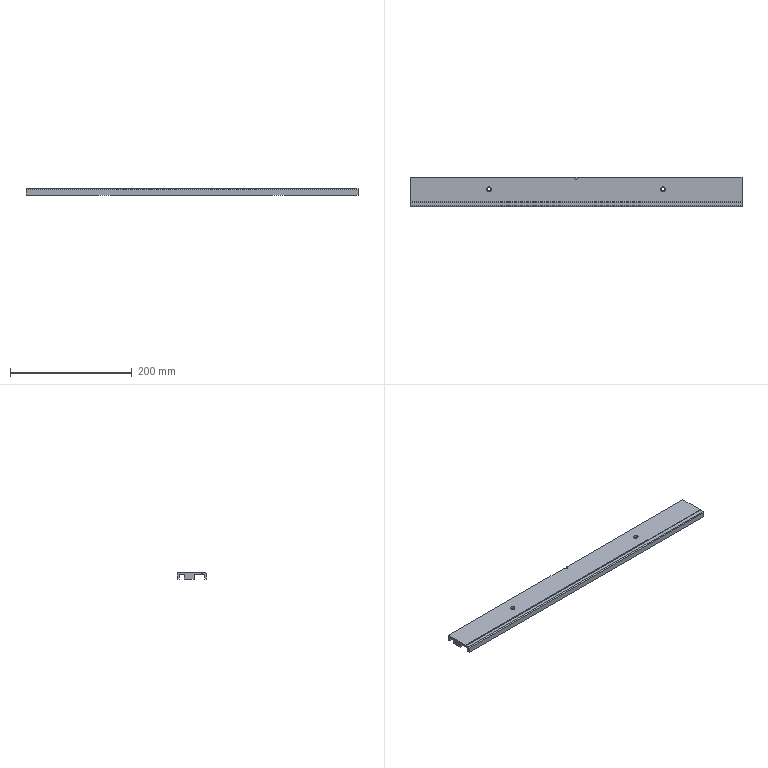Part | NX | features solid 2 | 1 solid | 39 faces | box 544.75 x 48.5 x 10 mm | volume 160065 mm3 | plane 30 | cylinder 9 | commonest cylinder face diameters 5.5 x4 8 x4 6.718 x1
STEP:
#1=CARTESIAN_POINT('',(272.5,-0.25,11.));
#2=VERTEX_POINT('',#1);
#3=CARTESIAN_POINT('',(272.5,-40.25,11.));
#4=VERTEX_POINT('',#3);
#5=CARTESIAN_POINT('',(272.5,-0.25,11.));
#6=DIRECTION('',(0.,-1.,0.));
#7=VECTOR('',#6,1000.);
#8=LINE('',#5,#7);
#9=EDGE_CURVE('',#2,#4,#8,.T.);
#10=ORIENTED_EDGE('',*,*,#9,.F.);
#11=CARTESIAN_POINT('',(3.484,-0.25,11.));
#12=VERTEX_POINT('',#11);
#13=CARTESIAN_POINT('',(3.484,-0.25,11.));
#14=DIRECTION('',(1.,0.,0.));
#15=VECTOR('',#14,1000.);
#16=LINE('',#13,#15);
#17=EDGE_CURVE('',#12,#2,#16,.T.);
#18=ORIENTED_EDGE('',*,*,#17,.F.);
#19=CARTESIAN_POINT('',(-3.234,-0.25,11.));
#20=VERTEX_POINT('',#19);
#21=CARTESIAN_POINT('',(0.125,-0.25,11.));
#22=DIRECTION('',(0.,0.,1.));
#23=DIRECTION('',(-1.,0.,0.));
#24=AXIS2_PLACEMENT_3D('',#21,#22,#23);
#25=CIRCLE('',#24,3.359);
#26=EDGE_CURVE('',#20,#12,#25,.T.);
#27=ORIENTED_EDGE('',*,*,#26,.F.);
#28=CARTESIAN_POINT('',(-272.25,-0.25,11.));
#29=VERTEX_POINT('',#28);
#30=CARTESIAN_POINT('',(-272.25,-0.25,11.));
#31=DIRECTION('',(1.,0.,0.));
#32=VECTOR('',#31,1000.);
#33=LINE('',#30,#32);
#34=EDGE_CURVE('',#29,#20,#33,.T.);
#35=ORIENTED_EDGE('',*,*,#34,.F.);
#36=CARTESIAN_POINT('',(-272.25,-40.25,11.));
#37=VERTEX_POINT('',#36);
#38=CARTESIAN_POINT('',(-272.25,-40.25,11.));
#39=DIRECTION('',(0.,1.,0.));
#40=VECTOR('',#39,1000.);
#41=LINE('',#38,#40);
#42=EDGE_CURVE('',#37,#29,#41,.T.);
#43=ORIENTED_EDGE('',*,*,#42,.F.);
#44=CARTESIAN_POINT('',(-272.25,-40.25,11.));
#45=DIRECTION('',(1.,0.,0.));
#46=VECTOR('',#45,1000.);
#47=LINE('',#44,#46);
#48=EDGE_CURVE('',#37,#4,#47,.T.);
#49=ORIENTED_EDGE('',*,*,#48,.T.);
#50=EDGE_LOOP('',(#10,#18,#27,#35,#43,#49));
#51=FACE_BOUND('',#50,.T.);
#52=CARTESIAN_POINT('',(-146.625,-20.,11.));
#53=VERTEX_POINT('',#52);
#54=CARTESIAN_POINT('',(-138.625,-20.,11.));
#55=VERTEX_POINT('',#54);
#56=CARTESIAN_POINT('',(-142.625,-20.,11.));
#57=DIRECTION('',(0.,0.,1.));
#58=DIRECTION('',(-1.,0.,0.));
#59=AXIS2_PLACEMENT_3D('',#56,#57,#58);
#60=CIRCLE('',#59,4.);
#61=EDGE_CURVE('',#53,#55,#60,.T.);
#62=ORIENTED_EDGE('',*,*,#61,.F.);
#63=CARTESIAN_POINT('',(-142.625,-20.,11.));
#64=DIRECTION('',(0.,0.,1.));
#65=DIRECTION('',(1.,0.,0.));
#66=AXIS2_PLACEMENT_3D('',#63,#64,#65);
#67=CIRCLE('',#66,4.);
#68=EDGE_CURVE('',#55,#53,#67,.T.);
#69=ORIENTED_EDGE('',*,*,#68,.F.);
#70=EDGE_LOOP('',(#62,#69));
#71=FACE_BOUND('',#70,.T.);
#72=CARTESIAN_POINT('',(138.875,-20.,11.));
#73=VERTEX_POINT('',#72);
#74=CARTESIAN_POINT('',(146.875,-20.,11.));
#75=VERTEX_POINT('',#74);
#76=CARTESIAN_POINT('',(142.875,-20.,11.));
#77=DIRECTION('',(0.,0.,1.));
#78=DIRECTION('',(-1.,0.,0.));
#79=AXIS2_PLACEMENT_3D('',#76,#77,#78);
#80=CIRCLE('',#79,4.);
#81=EDGE_CURVE('',#73,#75,#80,.T.);
#82=ORIENTED_EDGE('',*,*,#81,.F.);
#83=CARTESIAN_POINT('',(142.875,-20.,11.));
#84=DIRECTION('',(0.,0.,1.));
#85=DIRECTION('',(1.,0.,0.));
#86=AXIS2_PLACEMENT_3D('',#83,#84,#85);
#87=CIRCLE('',#86,4.);
#88=EDGE_CURVE('',#75,#73,#87,.T.);
#89=ORIENTED_EDGE('',*,*,#88,.F.);
#90=EDGE_LOOP('',(#82,#89));
#91=FACE_BOUND('',#90,.T.);
#92=CARTESIAN_POINT('',(0.125,-24.5,11.));
#93=DIRECTION('',(0.,0.,-1.));
#94=DIRECTION('',(-1.,0.,0.));
#95=AXIS2_PLACEMENT_3D('',#92,#93,#94);
#96=PLANE('',#95);
#97=ADVANCED_FACE('',(#51,#71,#91),#96,.F.);
#98=CARTESIAN_POINT('',(272.5,-41.75,11.));
#99=VERTEX_POINT('',#98);
#100=CARTESIAN_POINT('',(272.5,-47.25,11.));
#101=VERTEX_POINT('',#100);
#102=CARTESIAN_POINT('',(272.5,-41.75,11.));
#103=DIRECTION('',(0.,-1.,0.));
#104=VECTOR('',#103,1000.);
#105=LINE('',#102,#104);
#106=EDGE_CURVE('',#99,#101,#105,.T.);
#107=ORIENTED_EDGE('',*,*,#106,.F.);
#108=CARTESIAN_POINT('',(-272.25,-41.75,11.));
#109=VERTEX_POINT('',#108);
#110=CARTESIAN_POINT('',(-272.25,-41.75,11.));
#111=DIRECTION('',(1.,0.,0.));
#112=VECTOR('',#111,1000.);
#113=LINE('',#110,#112);
#114=EDGE_CURVE('',#109,#99,#113,.T.);
#115=ORIENTED_EDGE('',*,*,#114,.F.);
#116=CARTESIAN_POINT('',(-272.25,-47.25,11.));
#117=VERTEX_POINT('',#116);
#118=CARTESIAN_POINT('',(-272.25,-47.25,11.));
#119=DIRECTION('',(0.,1.,0.));
#120=VECTOR('',#119,1000.);
#121=LINE('',#118,#120);
#122=EDGE_CURVE('',#117,#109,#121,.T.);
#123=ORIENTED_EDGE('',*,*,#122,.F.);
#124=CARTESIAN_POINT('',(-272.25,-47.25,11.));
#125=DIRECTION('',(1.,0.,0.));
#126=VECTOR('',#125,1000.);
#127=LINE('',#124,#126);
#128=EDGE_CURVE('',#117,#101,#127,.T.);
#129=ORIENTED_EDGE('',*,*,#128,.T.);
#130=EDGE_LOOP('',(#107,#115,#123,#129));
#131=FACE_BOUND('',#130,.T.);
#132=CARTESIAN_POINT('',(0.125,-24.5,11.));
#133=DIRECTION('',(0.,0.,-1.));
#134=DIRECTION('',(-1.,0.,0.));
#135=AXIS2_PLACEMENT_3D('',#132,#133,#134);
#136=PLANE('',#135);
#137=ADVANCED_FACE('',(#131),#136,.F.);
#138=CARTESIAN_POINT('',(-146.625,-20.,7.));
#139=VERTEX_POINT('',#138);
#140=CARTESIAN_POINT('',(-146.625,-20.,11.));
#141=DIRECTION('',(0.,0.,-1.));
#142=VECTOR('',#141,1000.);
#143=LINE('',#140,#142);
#144=EDGE_CURVE('',#139,#53,#143,.F.);
#145=ORIENTED_EDGE('',*,*,#144,.F.);
#146=CARTESIAN_POINT('',(-138.625,-20.,7.));
#147=VERTEX_POINT('',#146);
#148=CARTESIAN_POINT('',(-142.625,-20.,7.));
#149=DIRECTION('',(0.,0.,1.));
#150=DIRECTION('',(1.,0.,0.));
#151=AXIS2_PLACEMENT_3D('',#148,#149,#150);
#152=CIRCLE('',#151,4.);
#153=EDGE_CURVE('',#147,#139,#152,.T.);
#154=ORIENTED_EDGE('',*,*,#153,.F.);
#155=CARTESIAN_POINT('',(-138.625,-20.,11.));
#156=DIRECTION('',(0.,0.,-1.));
#157=VECTOR('',#156,1000.);
#158=LINE('',#155,#157);
#159=EDGE_CURVE('',#55,#147,#158,.T.);
#160=ORIENTED_EDGE('',*,*,#159,.F.);
#161=ORIENTED_EDGE('',*,*,#68,.T.);
#162=EDGE_LOOP('',(#145,#154,#160,#161));
#163=FACE_BOUND('',#162,.T.);
#164=CARTESIAN_POINT('',(-142.625,-20.,11.));
#165=DIRECTION('',(0.,0.,1.));
#166=DIRECTION('',(-1.,0.,0.));
#167=AXIS2_PLACEMENT_3D('',#164,#165,#166);
#168=CYLINDRICAL_SURFACE('',#167,4.);
#169=ADVANCED_FACE('',(#163),#168,.F.);
#170=ORIENTED_EDGE('',*,*,#159,.T.);
#171=CARTESIAN_POINT('',(-142.625,-20.,7.));
#172=DIRECTION('',(0.,0.,1.));
#173=DIRECTION('',(-1.,0.,0.));
#174=AXIS2_PLACEMENT_3D('',#171,#172,#173);
#175=CIRCLE('',#174,4.);
#176=EDGE_CURVE('',#139,#147,#175,.T.);
#177=ORIENTED_EDGE('',*,*,#176,.F.);
#178=ORIENTED_EDGE('',*,*,#144,.T.);
#179=ORIENTED_EDGE('',*,*,#61,.T.);
#180=EDGE_LOOP('',(#170,#177,#178,#179));
#181=FACE_BOUND('',#180,.T.);
#182=CARTESIAN_POINT('',(-142.625,-20.,11.));
#183=DIRECTION('',(0.,0.,1.));
#184=DIRECTION('',(-1.,0.,0.));
#185=AXIS2_PLACEMENT_3D('',#182,#183,#184);
#186=CYLINDRICAL_SURFACE('',#185,4.);
#187=ADVANCED_FACE('',(#181),#186,.F.);
#188=ORIENTED_EDGE('',*,*,#176,.T.);
#189=ORIENTED_EDGE('',*,*,#153,.T.);
#190=EDGE_LOOP('',(#188,#189));
#191=FACE_BOUND('',#190,.T.);
#192=CARTESIAN_POINT('',(-145.375,-20.,7.));
#193=VERTEX_POINT('',#192);
#194=CARTESIAN_POINT('',(-139.875,-20.,7.));
#195=VERTEX_POINT('',#194);
#196=CARTESIAN_POINT('',(-142.625,-20.,7.));
#197=DIRECTION('',(0.,0.,1.));
#198=DIRECTION('',(-1.,0.,0.));
#199=AXIS2_PLACEMENT_3D('',#196,#197,#198);
#200=CIRCLE('',#199,2.75);
#201=EDGE_CURVE('',#193,#195,#200,.T.);
#202=ORIENTED_EDGE('',*,*,#201,.F.);
#203=CARTESIAN_POINT('',(-142.625,-20.,7.));
#204=DIRECTION('',(0.,0.,1.));
#205=DIRECTION('',(1.,0.,0.));
#206=AXIS2_PLACEMENT_3D('',#203,#204,#205);
#207=CIRCLE('',#206,2.75);
#208=EDGE_CURVE('',#195,#193,#207,.T.);
#209=ORIENTED_EDGE('',*,*,#208,.F.);
#210=EDGE_LOOP('',(#202,#209));
#211=FACE_BOUND('',#210,.T.);
#212=CARTESIAN_POINT('',(0.125,-24.5,7.));
#213=DIRECTION('',(0.,0.,1.));
#214=DIRECTION('',(-1.,0.,0.));
#215=AXIS2_PLACEMENT_3D('',#212,#213,#214);
#216=PLANE('',#215);
#217=ADVANCED_FACE('',(#191,#211),#216,.T.);
#218=CARTESIAN_POINT('',(138.875,-20.,7.));
#219=VERTEX_POINT('',#218);
#220=CARTESIAN_POINT('',(146.875,-20.,7.));
#221=VERTEX_POINT('',#220);
#222=CARTESIAN_POINT('',(142.875,-20.,7.));
#223=DIRECTION('',(0.,0.,1.));
#224=DIRECTION('',(-1.,0.,0.));
#225=AXIS2_PLACEMENT_3D('',#222,#223,#224);
#226=CIRCLE('',#225,4.);
#227=EDGE_CURVE('',#219,#221,#226,.T.);
#228=ORIENTED_EDGE('',*,*,#227,.T.);
#229=CARTESIAN_POINT('',(142.875,-20.,7.));
#230=DIRECTION('',(0.,0.,1.));
#231=DIRECTION('',(1.,0.,0.));
#232=AXIS2_PLACEMENT_3D('',#229,#230,#231);
#233=CIRCLE('',#232,4.);
#234=EDGE_CURVE('',#221,#219,#233,.T.);
#235=ORIENTED_EDGE('',*,*,#234,.T.);
#236=EDGE_LOOP('',(#228,#235));
#237=FACE_BOUND('',#236,.T.);
#238=CARTESIAN_POINT('',(140.125,-20.,7.));
#239=VERTEX_POINT('',#238);
#240=CARTESIAN_POINT('',(145.625,-20.,7.));
#241=VERTEX_POINT('',#240);
#242=CARTESIAN_POINT('',(142.875,-20.,7.));
#243=DIRECTION('',(0.,0.,1.));
#244=DIRECTION('',(-1.,0.,0.));
#245=AXIS2_PLACEMENT_3D('',#242,#243,#244);
#246=CIRCLE('',#245,2.75);
#247=EDGE_CURVE('',#239,#241,#246,.T.);
#248=ORIENTED_EDGE('',*,*,#247,.F.);
#249=CARTESIAN_POINT('',(142.875,-20.,7.));
#250=DIRECTION('',(0.,0.,1.));
#251=DIRECTION('',(1.,0.,0.));
#252=AXIS2_PLACEMENT_3D('',#249,#250,#251);
#253=CIRCLE('',#252,2.75);
#254=EDGE_CURVE('',#241,#239,#253,.T.);
#255=ORIENTED_EDGE('',*,*,#254,.F.);
#256=EDGE_LOOP('',(#248,#255));
#257=FACE_BOUND('',#256,.T.);
#258=CARTESIAN_POINT('',(0.125,-24.5,7.));
#259=DIRECTION('',(0.,0.,1.));
#260=DIRECTION('',(-1.,0.,0.));
#261=AXIS2_PLACEMENT_3D('',#258,#259,#260);
#262=PLANE('',#261);
#263=ADVANCED_FACE('',(#237,#257),#262,.T.);
#264=CARTESIAN_POINT('',(138.875,-20.,11.));
#265=DIRECTION('',(0.,0.,-1.));
#266=VECTOR('',#265,1000.);
#267=LINE('',#264,#266);
#268=EDGE_CURVE('',#73,#219,#267,.T.);
#269=ORIENTED_EDGE('',*,*,#268,.T.);
#270=ORIENTED_EDGE('',*,*,#234,.F.);
#271=CARTESIAN_POINT('',(146.875,-20.,11.));
#272=DIRECTION('',(0.,0.,-1.));
#273=VECTOR('',#272,1000.);
#274=LINE('',#271,#273);
#275=EDGE_CURVE('',#221,#75,#274,.F.);
#276=ORIENTED_EDGE('',*,*,#275,.T.);
#277=ORIENTED_EDGE('',*,*,#88,.T.);
#278=EDGE_LOOP('',(#269,#270,#276,#277));
#279=FACE_BOUND('',#278,.T.);
#280=CARTESIAN_POINT('',(142.875,-20.,11.));
#281=DIRECTION('',(0.,0.,1.));
#282=DIRECTION('',(-1.,0.,0.));
#283=AXIS2_PLACEMENT_3D('',#280,#281,#282);
#284=CYLINDRICAL_SURFACE('',#283,4.);
#285=ADVANCED_FACE('',(#279),#284,.F.);
#286=ORIENTED_EDGE('',*,*,#275,.F.);
#287=ORIENTED_EDGE('',*,*,#227,.F.);
#288=ORIENTED_EDGE('',*,*,#268,.F.);
#289=ORIENTED_EDGE('',*,*,#81,.T.);
#290=EDGE_LOOP('',(#286,#287,#288,#289));
#291=FACE_BOUND('',#290,.T.);
#292=CARTESIAN_POINT('',(142.875,-20.,11.));
#293=DIRECTION('',(0.,0.,1.));
#294=DIRECTION('',(-1.,0.,0.));
#295=AXIS2_PLACEMENT_3D('',#292,#293,#294);
#296=CYLINDRICAL_SURFACE('',#295,4.);
#297=ADVANCED_FACE('',(#291),#296,.F.);
#298=CARTESIAN_POINT('',(-139.875,-20.,2.5));
#299=VERTEX_POINT('',#298);
#300=CARTESIAN_POINT('',(-139.875,-20.,7.));
#301=DIRECTION('',(0.,0.,-1.));
#302=VECTOR('',#301,1000.);
#303=LINE('',#300,#302);
#304=EDGE_CURVE('',#299,#195,#303,.F.);
#305=ORIENTED_EDGE('',*,*,#304,.T.);
#306=ORIENTED_EDGE('',*,*,#208,.T.);
#307=CARTESIAN_POINT('',(-145.375,-20.,2.5));
#308=VERTEX_POINT('',#307);
#309=CARTESIAN_POINT('',(-145.375,-20.,7.));
#310=DIRECTION('',(0.,0.,-1.));
#311=VECTOR('',#310,1000.);
#312=LINE('',#309,#311);
#313=EDGE_CURVE('',#193,#308,#312,.T.);
#314=ORIENTED_EDGE('',*,*,#313,.T.);
#315=CARTESIAN_POINT('',(-142.625,-20.,2.5));
#316=DIRECTION('',(0.,0.,1.));
#317=DIRECTION('',(1.,0.,0.));
#318=AXIS2_PLACEMENT_3D('',#315,#316,#317);
#319=CIRCLE('',#318,2.75);
#320=EDGE_CURVE('',#299,#308,#319,.T.);
#321=ORIENTED_EDGE('',*,*,#320,.F.);
#322=EDGE_LOOP('',(#305,#306,#314,#321));
#323=FACE_BOUND('',#322,.T.);
#324=CARTESIAN_POINT('',(-142.625,-20.,11.));
#325=DIRECTION('',(0.,0.,1.));
#326=DIRECTION('',(-1.,0.,0.));
#327=AXIS2_PLACEMENT_3D('',#324,#325,#326);
#328=CYLINDRICAL_SURFACE('',#327,2.75);
#329=ADVANCED_FACE('',(#323),#328,.F.);
#330=CARTESIAN_POINT('',(153.361,-12.,2.5));
#331=VERTEX_POINT('',#330);
#332=CARTESIAN_POINT('',(153.361,-28.,2.5));
#333=VERTEX_POINT('',#332);
#334=CARTESIAN_POINT('',(153.361,-12.,2.5));
#335=DIRECTION('',(0.,-1.,0.));
#336=VECTOR('',#335,1000.);
#337=LINE('',#334,#336);
#338=EDGE_CURVE('',#331,#333,#337,.T.);
#339=ORIENTED_EDGE('',*,*,#338,.T.);
#340=CARTESIAN_POINT('',(132.389,-28.,2.5));
#341=VERTEX_POINT('',#340);
#342=CARTESIAN_POINT('',(153.361,-28.,2.5));
#343=DIRECTION('',(-1.,0.,0.));
#344=VECTOR('',#343,1000.);
#345=LINE('',#342,#344);
#346=EDGE_CURVE('',#333,#341,#345,.T.);
#347=ORIENTED_EDGE('',*,*,#346,.T.);
#348=CARTESIAN_POINT('',(132.389,-12.,2.5));
#349=VERTEX_POINT('',#348);
#350=CARTESIAN_POINT('',(132.389,-28.,2.5));
#351=DIRECTION('',(0.,1.,0.));
#352=VECTOR('',#351,1000.);
#353=LINE('',#350,#352);
#354=EDGE_CURVE('',#341,#349,#353,.T.);
#355=ORIENTED_EDGE('',*,*,#354,.T.);
#356=CARTESIAN_POINT('',(153.361,-12.,2.5));
#357=DIRECTION('',(-1.,0.,0.));
#358=VECTOR('',#357,1000.);
#359=LINE('',#356,#358);
#360=EDGE_CURVE('',#331,#349,#359,.T.);
#361=ORIENTED_EDGE('',*,*,#360,.F.);
#362=EDGE_LOOP('',(#339,#347,#355,#361));
#363=FACE_BOUND('',#362,.T.);
#364=CARTESIAN_POINT('',(140.125,-20.,2.5));
#365=VERTEX_POINT('',#364);
#366=CARTESIAN_POINT('',(145.625,-20.,2.5));
#367=VERTEX_POINT('',#366);
#368=CARTESIAN_POINT('',(142.875,-20.,2.5));
#369=DIRECTION('',(0.,0.,1.));
#370=DIRECTION('',(-1.,0.,0.));
#371=AXIS2_PLACEMENT_3D('',#368,#369,#370);
#372=CIRCLE('',#371,2.75);
#373=EDGE_CURVE('',#365,#367,#372,.T.);
#374=ORIENTED_EDGE('',*,*,#373,.T.);
#375=CARTESIAN_POINT('',(142.875,-20.,2.5));
#376=DIRECTION('',(0.,0.,1.));
#377=DIRECTION('',(1.,0.,0.));
#378=AXIS2_PLACEMENT_3D('',#375,#376,#377);
#379=CIRCLE('',#378,2.75);
#380=EDGE_CURVE('',#367,#365,#379,.T.);
#381=ORIENTED_EDGE('',*,*,#380,.T.);
#382=EDGE_LOOP('',(#374,#381));
#383=FACE_BOUND('',#382,.T.);
#384=CARTESIAN_POINT('',(0.125,-24.5,2.5));
#385=DIRECTION('',(0.,0.,-1.));
#386=DIRECTION('',(1.,0.,0.));
#387=AXIS2_PLACEMENT_3D('',#384,#385,#386);
#388=PLANE('',#387);
#389=ADVANCED_FACE('',(#363,#383),#388,.T.);
#390=CARTESIAN_POINT('',(-132.139,-12.,2.5));
#391=VERTEX_POINT('',#390);
#392=CARTESIAN_POINT('',(-132.139,-28.,2.5));
#393=VERTEX_POINT('',#392);
#394=CARTESIAN_POINT('',(-132.139,-12.,2.5));
#395=DIRECTION('',(0.,-1.,0.));
#396=VECTOR('',#395,1000.);
#397=LINE('',#394,#396);
#398=EDGE_CURVE('',#391,#393,#397,.T.);
#399=ORIENTED_EDGE('',*,*,#398,.T.);
#400=CARTESIAN_POINT('',(-153.111,-28.,2.5));
#401=VERTEX_POINT('',#400);
#402=CARTESIAN_POINT('',(-132.139,-28.,2.5));
#403=DIRECTION('',(-1.,0.,0.));
#404=VECTOR('',#403,1000.);
#405=LINE('',#402,#404);
#406=EDGE_CURVE('',#393,#401,#405,.T.);
#407=ORIENTED_EDGE('',*,*,#406,.T.);
#408=CARTESIAN_POINT('',(-153.111,-12.,2.5));
#409=VERTEX_POINT('',#408);
#410=CARTESIAN_POINT('',(-153.111,-28.,2.5));
#411=DIRECTION('',(0.,1.,0.));
#412=VECTOR('',#411,1000.);
#413=LINE('',#410,#412);
#414=EDGE_CURVE('',#401,#409,#413,.T.);
#415=ORIENTED_EDGE('',*,*,#414,.T.);
#416=CARTESIAN_POINT('',(-132.139,-12.,2.5));
#417=DIRECTION('',(-1.,0.,0.));
#418=VECTOR('',#417,1000.);
#419=LINE('',#416,#418);
#420=EDGE_CURVE('',#391,#409,#419,.T.);
#421=ORIENTED_EDGE('',*,*,#420,.F.);
#422=EDGE_LOOP('',(#399,#407,#415,#421));
#423=FACE_BOUND('',#422,.T.);
#424=CARTESIAN_POINT('',(-142.625,-20.,2.5));
#425=DIRECTION('',(0.,0.,1.));
#426=DIRECTION('',(-1.,0.,0.));
#427=AXIS2_PLACEMENT_3D('',#424,#425,#426);
#428=CIRCLE('',#427,2.75);
#429=EDGE_CURVE('',#308,#299,#428,.T.);
#430=ORIENTED_EDGE('',*,*,#429,.T.);
#431=ORIENTED_EDGE('',*,*,#320,.T.);
#432=EDGE_LOOP('',(#430,#431));
#433=FACE_BOUND('',#432,.T.);
#434=CARTESIAN_POINT('',(0.125,-24.5,2.5));
#435=DIRECTION('',(0.,0.,-1.));
#436=DIRECTION('',(1.,0.,0.));
#437=AXIS2_PLACEMENT_3D('',#434,#435,#436);
#438=PLANE('',#437);
#439=ADVANCED_FACE('',(#423,#433),#438,.T.);
#440=ORIENTED_EDGE('',*,*,#313,.F.);
#441=ORIENTED_EDGE('',*,*,#201,.T.);
#442=ORIENTED_EDGE('',*,*,#304,.F.);
#443=ORIENTED_EDGE('',*,*,#429,.F.);
#444=EDGE_LOOP('',(#440,#441,#442,#443));
#445=FACE_BOUND('',#444,.T.);
#446=CARTESIAN_POINT('',(-142.625,-20.,11.));
#447=DIRECTION('',(0.,0.,1.));
#448=DIRECTION('',(-1.,0.,0.));
#449=AXIS2_PLACEMENT_3D('',#446,#447,#448);
#450=CYLINDRICAL_SURFACE('',#449,2.75);
#451=ADVANCED_FACE('',(#445),#450,.F.);
#452=CARTESIAN_POINT('',(145.625,-20.,7.));
#453=DIRECTION('',(0.,0.,-1.));
#454=VECTOR('',#453,1000.);
#455=LINE('',#452,#454);
#456=EDGE_CURVE('',#241,#367,#455,.T.);
#457=ORIENTED_EDGE('',*,*,#456,.F.);
#458=ORIENTED_EDGE('',*,*,#254,.T.);
#459=CARTESIAN_POINT('',(140.125,-20.,7.));
#460=DIRECTION('',(0.,0.,-1.));
#461=VECTOR('',#460,1000.);
#462=LINE('',#459,#461);
#463=EDGE_CURVE('',#365,#239,#462,.F.);
#464=ORIENTED_EDGE('',*,*,#463,.F.);
#465=ORIENTED_EDGE('',*,*,#380,.F.);
#466=EDGE_LOOP('',(#457,#458,#464,#465));
#467=FACE_BOUND('',#466,.T.);
#468=CARTESIAN_POINT('',(142.875,-20.,11.));
#469=DIRECTION('',(0.,0.,1.));
#470=DIRECTION('',(-1.,0.,0.));
#471=AXIS2_PLACEMENT_3D('',#468,#469,#470);
#472=CYLINDRICAL_SURFACE('',#471,2.75);
#473=ADVANCED_FACE('',(#467),#472,.F.);
#474=ORIENTED_EDGE('',*,*,#463,.T.);
#475=ORIENTED_EDGE('',*,*,#247,.T.);
#476=ORIENTED_EDGE('',*,*,#456,.T.);
#477=ORIENTED_EDGE('',*,*,#373,.F.);
#478=EDGE_LOOP('',(#474,#475,#476,#477));
#479=FACE_BOUND('',#478,.T.);
#480=CARTESIAN_POINT('',(142.875,-20.,11.));
#481=DIRECTION('',(0.,0.,1.));
#482=DIRECTION('',(-1.,0.,0.));
#483=AXIS2_PLACEMENT_3D('',#480,#481,#482);
#484=CYLINDRICAL_SURFACE('',#483,2.75);
#485=ADVANCED_FACE('',(#479),#484,.F.);
#486=CARTESIAN_POINT('',(132.389,-12.,1.));
#487=VERTEX_POINT('',#486);
#488=CARTESIAN_POINT('',(132.389,-12.,1.));
#489=DIRECTION('',(0.,0.,1.));
#490=VECTOR('',#489,1000.);
#491=LINE('',#488,#490);
#492=EDGE_CURVE('',#487,#349,#491,.T.);
#493=ORIENTED_EDGE('',*,*,#492,.F.);
#494=CARTESIAN_POINT('',(-132.139,-12.,1.));
#495=VERTEX_POINT('',#494);
#496=CARTESIAN_POINT('',(-132.139,-12.,1.));
#497=DIRECTION('',(1.,0.,0.));
#498=VECTOR('',#497,1000.);
#499=LINE('',#496,#498);
#500=EDGE_CURVE('',#495,#487,#499,.T.);
#501=ORIENTED_EDGE('',*,*,#500,.F.);
#502=CARTESIAN_POINT('',(-132.139,-12.,1.));
#503=DIRECTION('',(0.,0.,1.));
#504=VECTOR('',#503,1000.);
#505=LINE('',#502,#504);
#506=EDGE_CURVE('',#495,#391,#505,.T.);
#507=ORIENTED_EDGE('',*,*,#506,.T.);
#508=ORIENTED_EDGE('',*,*,#420,.T.);
#509=CARTESIAN_POINT('',(-153.111,-12.,1.));
#510=VERTEX_POINT('',#509);
#511=CARTESIAN_POINT('',(-153.111,-12.,1.));
#512=DIRECTION('',(0.,0.,1.));
#513=VECTOR('',#512,1000.);
#514=LINE('',#511,#513);
#515=EDGE_CURVE('',#510,#409,#514,.T.);
#516=ORIENTED_EDGE('',*,*,#515,.F.);
#517=CARTESIAN_POINT('',(-272.25,-12.,1.));
#518=VERTEX_POINT('',#517);
#519=CARTESIAN_POINT('',(-272.25,-12.,1.));
#520=DIRECTION('',(1.,0.,0.));
#521=VECTOR('',#520,1000.);
#522=LINE('',#519,#521);
#523=EDGE_CURVE('',#518,#510,#522,.T.);
#524=ORIENTED_EDGE('',*,*,#523,.F.);
#525=CARTESIAN_POINT('',(-272.25,-12.,8.));
#526=VERTEX_POINT('',#525);
#527=CARTESIAN_POINT('',(-272.25,-12.,1.));
#528=DIRECTION('',(0.,0.,1.));
#529=VECTOR('',#528,1000.);
#530=LINE('',#527,#529);
#531=EDGE_CURVE('',#518,#526,#530,.T.);
#532=ORIENTED_EDGE('',*,*,#531,.T.);
#533=CARTESIAN_POINT('',(272.5,-12.,8.));
#534=VERTEX_POINT('',#533);
#535=CARTESIAN_POINT('',(-272.25,-12.,8.));
#536=DIRECTION('',(1.,0.,0.));
#537=VECTOR('',#536,1000.);
#538=LINE('',#535,#537);
#539=EDGE_CURVE('',#526,#534,#538,.T.);
#540=ORIENTED_EDGE('',*,*,#539,.T.);
#541=CARTESIAN_POINT('',(272.5,-12.,1.));
#542=VERTEX_POINT('',#541);
#543=CARTESIAN_POINT('',(272.5,-12.,1.));
#544=DIRECTION('',(0.,0.,1.));
#545=VECTOR('',#544,1000.);
#546=LINE('',#543,#545);
#547=EDGE_CURVE('',#542,#534,#546,.T.);
#548=ORIENTED_EDGE('',*,*,#547,.F.);
#549=CARTESIAN_POINT('',(153.361,-12.,1.));
#550=VERTEX_POINT('',#549);
#551=CARTESIAN_POINT('',(153.361,-12.,1.));
#552=DIRECTION('',(1.,0.,0.));
#553=VECTOR('',#552,1000.);
#554=LINE('',#551,#553);
#555=EDGE_CURVE('',#550,#542,#554,.T.);
#556=ORIENTED_EDGE('',*,*,#555,.F.);
#557=CARTESIAN_POINT('',(153.361,-12.,1.));
#558=DIRECTION('',(0.,0.,1.));
#559=VECTOR('',#558,1000.);
#560=LINE('',#557,#559);
#561=EDGE_CURVE('',#550,#331,#560,.T.);
#562=ORIENTED_EDGE('',*,*,#561,.T.);
#563=ORIENTED_EDGE('',*,*,#360,.T.);
#564=EDGE_LOOP('',(#493,#501,#507,#508,#516,#524,#532,#540,#548,#556,#562,#563));
#565=FACE_BOUND('',#564,.T.);
#566=CARTESIAN_POINT('',(-272.25,-12.,1.));
#567=DIRECTION('',(0.,-1.,0.));
#568=DIRECTION('',(0.,0.,-1.));
#569=AXIS2_PLACEMENT_3D('',#566,#567,#568);
#570=PLANE('',#569);
#571=ADVANCED_FACE('',(#565),#570,.F.);
#572=CARTESIAN_POINT('',(153.361,-28.,1.));
#573=VERTEX_POINT('',#572);
#574=CARTESIAN_POINT('',(153.361,-28.,1.));
#575=DIRECTION('',(0.,0.,1.));
#576=VECTOR('',#575,1000.);
#577=LINE('',#574,#576);
#578=EDGE_CURVE('',#573,#333,#577,.T.);
#579=ORIENTED_EDGE('',*,*,#578,.T.);
#580=ORIENTED_EDGE('',*,*,#338,.F.);
#581=ORIENTED_EDGE('',*,*,#561,.F.);
#582=CARTESIAN_POINT('',(153.361,-12.,1.));
#583=DIRECTION('',(0.,-1.,0.));
#584=VECTOR('',#583,1000.);
#585=LINE('',#582,#584);
#586=EDGE_CURVE('',#550,#573,#585,.T.);
#587=ORIENTED_EDGE('',*,*,#586,.T.);
#588=EDGE_LOOP('',(#579,#580,#581,#587));
#589=FACE_BOUND('',#588,.T.);
#590=CARTESIAN_POINT('',(153.361,-12.,1.));
#591=DIRECTION('',(1.,0.,0.));
#592=DIRECTION('',(0.,1.,0.));
#593=AXIS2_PLACEMENT_3D('',#590,#591,#592);
#594=PLANE('',#593);
#595=ADVANCED_FACE('',(#589),#594,.F.);
#596=CARTESIAN_POINT('',(-272.25,-3.25,1.));
#597=VERTEX_POINT('',#596);
#598=CARTESIAN_POINT('',(-272.25,-0.25,1.));
#599=VERTEX_POINT('',#598);
#600=CARTESIAN_POINT('',(-272.25,-3.25,1.));
#601=DIRECTION('',(0.,1.,0.));
#602=VECTOR('',#601,1000.);
#603=LINE('',#600,#602);
#604=EDGE_CURVE('',#597,#599,#603,.T.);
#605=ORIENTED_EDGE('',*,*,#604,.T.);
#606=CARTESIAN_POINT('',(272.5,-0.25,1.));
#607=VERTEX_POINT('',#606);
#608=CARTESIAN_POINT('',(-272.25,-0.25,1.));
#609=DIRECTION('',(1.,0.,0.));
#610=VECTOR('',#609,1000.);
#611=LINE('',#608,#610);
#612=EDGE_CURVE('',#599,#607,#611,.T.);
#613=ORIENTED_EDGE('',*,*,#612,.T.);
#614=CARTESIAN_POINT('',(272.5,-3.25,1.));
#615=VERTEX_POINT('',#614);
#616=CARTESIAN_POINT('',(272.5,-0.25,1.));
#617=DIRECTION('',(0.,-1.,0.));
#618=VECTOR('',#617,1000.);
#619=LINE('',#616,#618);
#620=EDGE_CURVE('',#607,#615,#619,.T.);
#621=ORIENTED_EDGE('',*,*,#620,.T.);
#622=CARTESIAN_POINT('',(-272.25,-3.25,1.));
#623=DIRECTION('',(1.,0.,0.));
#624=VECTOR('',#623,1000.);
#625=LINE('',#622,#624);
#626=EDGE_CURVE('',#597,#615,#625,.T.);
#627=ORIENTED_EDGE('',*,*,#626,.F.);
#628=EDGE_LOOP('',(#605,#613,#621,#627));
#629=FACE_BOUND('',#628,.T.);
#630=CARTESIAN_POINT('',(0.125,-24.5,1.));
#631=DIRECTION('',(0.,0.,-1.));
#632=DIRECTION('',(-1.,0.,0.));
#633=AXIS2_PLACEMENT_3D('',#630,#631,#632);
#634=PLANE('',#633);
#635=ADVANCED_FACE('',(#629),#634,.T.);
#636=CARTESIAN_POINT('',(272.5,-45.75,1.));
#637=VERTEX_POINT('',#636);
#638=CARTESIAN_POINT('',(272.5,-48.75,1.));
#639=VERTEX_POINT('',#638);
#640=CARTESIAN_POINT('',(272.5,-45.75,1.));
#641=DIRECTION('',(0.,-1.,0.));
#642=VECTOR('',#641,1000.);
#643=LINE('',#640,#642);
#644=EDGE_CURVE('',#637,#639,#643,.T.);
#645=ORIENTED_EDGE('',*,*,#644,.T.);
#646=CARTESIAN_POINT('',(-272.25,-48.75,1.));
#647=VERTEX_POINT('',#646);
#648=CARTESIAN_POINT('',(272.5,-48.75,1.));
#649=DIRECTION('',(-1.,0.,0.));
#650=VECTOR('',#649,1000.);
#651=LINE('',#648,#650);
#652=EDGE_CURVE('',#639,#647,#651,.T.);
#653=ORIENTED_EDGE('',*,*,#652,.T.);
#654=CARTESIAN_POINT('',(-272.25,-45.75,1.));
#655=VERTEX_POINT('',#654);
#656=CARTESIAN_POINT('',(-272.25,-48.75,1.));
#657=DIRECTION('',(0.,1.,0.));
#658=VECTOR('',#657,1000.);
#659=LINE('',#656,#658);
#660=EDGE_CURVE('',#647,#655,#659,.T.);
#661=ORIENTED_EDGE('',*,*,#660,.T.);
#662=CARTESIAN_POINT('',(-272.25,-45.75,1.));
#663=DIRECTION('',(1.,0.,0.));
#664=VECTOR('',#663,1000.);
#665=LINE('',#662,#664);
#666=EDGE_CURVE('',#655,#637,#665,.T.);
#667=ORIENTED_EDGE('',*,*,#666,.T.);
#668=EDGE_LOOP('',(#645,#653,#661,#667));
#669=FACE_BOUND('',#668,.T.);
#670=CARTESIAN_POINT('',(0.125,-24.5,1.));
#671=DIRECTION('',(0.,0.,-1.));
#672=DIRECTION('',(-1.,0.,0.));
#673=AXIS2_PLACEMENT_3D('',#670,#671,#672);
#674=PLANE('',#673);
#675=ADVANCED_FACE('',(#669),#674,.T.);
#676=CARTESIAN_POINT('',(-132.139,-28.,1.));
#677=VERTEX_POINT('',#676);
#678=CARTESIAN_POINT('',(132.389,-28.,1.));
#679=VERTEX_POINT('',#678);
#680=CARTESIAN_POINT('',(-132.139,-28.,1.));
#681=DIRECTION('',(1.,0.,0.));
#682=VECTOR('',#681,1000.);
#683=LINE('',#680,#682);
#684=EDGE_CURVE('',#677,#679,#683,.T.);
#685=ORIENTED_EDGE('',*,*,#684,.F.);
#686=CARTESIAN_POINT('',(-132.139,-12.,1.));
#687=DIRECTION('',(0.,-1.,0.));
#688=VECTOR('',#687,1000.);
#689=LINE('',#686,#688);
#690=EDGE_CURVE('',#495,#677,#689,.T.);
#691=ORIENTED_EDGE('',*,*,#690,.F.);
#692=ORIENTED_EDGE('',*,*,#500,.T.);
#693=CARTESIAN_POINT('',(132.389,-28.,1.));
#694=DIRECTION('',(0.,1.,0.));
#695=VECTOR('',#694,1000.);
#696=LINE('',#693,#695);
#697=EDGE_CURVE('',#679,#487,#696,.T.);
#698=ORIENTED_EDGE('',*,*,#697,.F.);
#699=EDGE_LOOP('',(#685,#691,#692,#698));
#700=FACE_BOUND('',#699,.T.);
#701=CARTESIAN_POINT('',(0.125,-24.5,1.));
#702=DIRECTION('',(0.,0.,-1.));
#703=DIRECTION('',(-1.,0.,0.));
#704=AXIS2_PLACEMENT_3D('',#701,#702,#703);
#705=PLANE('',#704);
#706=ADVANCED_FACE('',(#700),#705,.T.);
#707=ORIENTED_EDGE('',*,*,#555,.T.);
#708=CARTESIAN_POINT('',(272.5,-28.,1.));
#709=VERTEX_POINT('',#708);
#710=CARTESIAN_POINT('',(272.5,-12.,1.));
#711=DIRECTION('',(0.,-1.,0.));
#712=VECTOR('',#711,1000.);
#713=LINE('',#710,#712);
#714=EDGE_CURVE('',#542,#709,#713,.T.);
#715=ORIENTED_EDGE('',*,*,#714,.T.);
#716=CARTESIAN_POINT('',(153.361,-28.,1.));
#717=DIRECTION('',(1.,0.,0.));
#718=VECTOR('',#717,1000.);
#719=LINE('',#716,#718);
#720=EDGE_CURVE('',#573,#709,#719,.T.);
#721=ORIENTED_EDGE('',*,*,#720,.F.);
#722=ORIENTED_EDGE('',*,*,#586,.F.);
#723=EDGE_LOOP('',(#707,#715,#721,#722));
#724=FACE_BOUND('',#723,.T.);
#725=CARTESIAN_POINT('',(0.125,-24.5,1.));
#726=DIRECTION('',(0.,0.,-1.));
#727=DIRECTION('',(-1.,0.,0.));
#728=AXIS2_PLACEMENT_3D('',#725,#726,#727);
#729=PLANE('',#728);
#730=ADVANCED_FACE('',(#724),#729,.T.);
#731=CARTESIAN_POINT('',(-272.25,-28.,1.));
#732=VERTEX_POINT('',#731);
#733=CARTESIAN_POINT('',(-153.111,-28.,1.));
#734=VERTEX_POINT('',#733);
#735=CARTESIAN_POINT('',(-272.25,-28.,1.));
#736=DIRECTION('',(1.,0.,0.));
#737=VECTOR('',#736,1000.);
#738=LINE('',#735,#737);
#739=EDGE_CURVE('',#732,#734,#738,.T.);
#740=ORIENTED_EDGE('',*,*,#739,.F.);
#741=CARTESIAN_POINT('',(-272.25,-28.,1.));
#742=DIRECTION('',(0.,1.,0.));
#743=VECTOR('',#742,1000.);
#744=LINE('',#741,#743);
#745=EDGE_CURVE('',#732,#518,#744,.T.);
#746=ORIENTED_EDGE('',*,*,#745,.T.);
#747=ORIENTED_EDGE('',*,*,#523,.T.);
#748=CARTESIAN_POINT('',(-153.111,-28.,1.));
#749=DIRECTION('',(0.,1.,0.));
#750=VECTOR('',#749,1000.);
#751=LINE('',#748,#750);
#752=EDGE_CURVE('',#734,#510,#751,.T.);
#753=ORIENTED_EDGE('',*,*,#752,.F.);
#754=EDGE_LOOP('',(#740,#746,#747,#753));
#755=FACE_BOUND('',#754,.T.);
#756=CARTESIAN_POINT('',(0.125,-24.5,1.));
#757=DIRECTION('',(0.,0.,-1.));
#758=DIRECTION('',(-1.,0.,0.));
#759=AXIS2_PLACEMENT_3D('',#756,#757,#758);
#760=PLANE('',#759);
#761=ADVANCED_FACE('',(#755),#760,.T.);
#762=CARTESIAN_POINT('',(272.5,-3.25,8.));
#763=VERTEX_POINT('',#762);
#764=CARTESIAN_POINT('',(272.5,-3.25,1.));
#765=DIRECTION('',(0.,0.,1.));
#766=VECTOR('',#765,1000.);
#767=LINE('',#764,#766);
#768=EDGE_CURVE('',#615,#763,#767,.T.);
#769=ORIENTED_EDGE('',*,*,#768,.T.);
#770=CARTESIAN_POINT('',(-272.25,-3.25,8.));
#771=VERTEX_POINT('',#770);
#772=CARTESIAN_POINT('',(-272.25,-3.25,8.));
#773=DIRECTION('',(1.,0.,0.));
#774=VECTOR('',#773,1000.);
#775=LINE('',#772,#774);
#776=EDGE_CURVE('',#771,#763,#775,.T.);
#777=ORIENTED_EDGE('',*,*,#776,.F.);
#778=CARTESIAN_POINT('',(-272.25,-3.25,1.));
#779=DIRECTION('',(0.,0.,1.));
#780=VECTOR('',#779,1000.);
#781=LINE('',#778,#780);
#782=EDGE_CURVE('',#597,#771,#781,.T.);
#783=ORIENTED_EDGE('',*,*,#782,.F.);
#784=ORIENTED_EDGE('',*,*,#626,.T.);
#785=EDGE_LOOP('',(#769,#777,#783,#784));
#786=FACE_BOUND('',#785,.T.);
#787=CARTESIAN_POINT('',(-272.25,-3.25,8.));
#788=DIRECTION('',(0.,1.,0.));
#789=DIRECTION('',(0.,0.,1.));
#790=AXIS2_PLACEMENT_3D('',#787,#788,#789);
#791=PLANE('',#790);
#792=ADVANCED_FACE('',(#786),#791,.F.);
#793=ORIENTED_EDGE('',*,*,#122,.T.);
#794=CARTESIAN_POINT('',(-272.25,-41.75,10.));
#795=VERTEX_POINT('',#794);
#796=CARTESIAN_POINT('',(-272.25,-41.75,11.));
#797=DIRECTION('',(0.,0.,-1.));
#798=VECTOR('',#797,1000.);
#799=LINE('',#796,#798);
#800=EDGE_CURVE('',#109,#795,#799,.T.);
#801=ORIENTED_EDGE('',*,*,#800,.T.);
#802=CARTESIAN_POINT('',(-272.25,-40.25,10.));
#803=VERTEX_POINT('',#802);
#804=CARTESIAN_POINT('',(-272.25,-41.75,10.));
#805=DIRECTION('',(0.,1.,0.));
#806=VECTOR('',#805,1000.);
#807=LINE('',#804,#806);
#808=EDGE_CURVE('',#795,#803,#807,.T.);
#809=ORIENTED_EDGE('',*,*,#808,.T.);
#810=CARTESIAN_POINT('',(-272.25,-40.25,11.));
#811=DIRECTION('',(0.,0.,-1.));
#812=VECTOR('',#811,1000.);
#813=LINE('',#810,#812);
#814=EDGE_CURVE('',#37,#803,#813,.T.);
#815=ORIENTED_EDGE('',*,*,#814,.F.);
#816=ORIENTED_EDGE('',*,*,#42,.T.);
#817=CARTESIAN_POINT('',(-272.25,-0.25,11.));
#818=DIRECTION('',(0.,0.,-1.));
#819=VECTOR('',#818,1000.);
#820=LINE('',#817,#819);
#821=EDGE_CURVE('',#29,#599,#820,.T.);
#822=ORIENTED_EDGE('',*,*,#821,.T.);
#823=ORIENTED_EDGE('',*,*,#604,.F.);
#824=ORIENTED_EDGE('',*,*,#782,.T.);
#825=CARTESIAN_POINT('',(-272.25,-12.,8.));
#826=DIRECTION('',(0.,1.,0.));
#827=VECTOR('',#826,1000.);
#828=LINE('',#825,#827);
#829=EDGE_CURVE('',#526,#771,#828,.T.);
#830=ORIENTED_EDGE('',*,*,#829,.F.);
#831=ORIENTED_EDGE('',*,*,#531,.F.);
#832=ORIENTED_EDGE('',*,*,#745,.F.);
#833=CARTESIAN_POINT('',(-272.25,-28.,8.));
#834=VERTEX_POINT('',#833);
#835=CARTESIAN_POINT('',(-272.25,-28.,1.));
#836=DIRECTION('',(0.,0.,1.));
#837=VECTOR('',#836,1000.);
#838=LINE('',#835,#837);
#839=EDGE_CURVE('',#732,#834,#838,.T.);
#840=ORIENTED_EDGE('',*,*,#839,.T.);
#841=CARTESIAN_POINT('',(-272.25,-45.75,8.));
#842=VERTEX_POINT('',#841);
#843=CARTESIAN_POINT('',(-272.25,-45.75,8.));
#844=DIRECTION('',(0.,1.,0.));
#845=VECTOR('',#844,1000.);
#846=LINE('',#843,#845);
#847=EDGE_CURVE('',#842,#834,#846,.T.);
#848=ORIENTED_EDGE('',*,*,#847,.F.);
#849=CARTESIAN_POINT('',(-272.25,-45.75,1.));
#850=DIRECTION('',(0.,0.,1.));
#851=VECTOR('',#850,1000.);
#852=LINE('',#849,#851);
#853=EDGE_CURVE('',#655,#842,#852,.T.);
#854=ORIENTED_EDGE('',*,*,#853,.F.);
#855=ORIENTED_EDGE('',*,*,#660,.F.);
#856=CARTESIAN_POINT('',(-272.25,-48.75,9.5));
#857=VERTEX_POINT('',#856);
#858=CARTESIAN_POINT('',(-272.25,-48.75,9.5));
#859=DIRECTION('',(0.,0.,-1.));
#860=VECTOR('',#859,1000.);
#861=LINE('',#858,#860);
#862=EDGE_CURVE('',#857,#647,#861,.T.);
#863=ORIENTED_EDGE('',*,*,#862,.F.);
#864=CARTESIAN_POINT('',(-272.25,-48.75,9.5));
#865=DIRECTION('',(0.,0.7071,0.7071));
#866=VECTOR('',#865,1000.);
#867=LINE('',#864,#866);
#868=EDGE_CURVE('',#857,#117,#867,.T.);
#869=ORIENTED_EDGE('',*,*,#868,.T.);
#870=EDGE_LOOP('',(#793,#801,#809,#815,#816,#822,#823,#824,#830,#831,#832,#840,#848,#854,#855,#863,#869));
#871=FACE_BOUND('',#870,.T.);
#872=CARTESIAN_POINT('',(-272.25,-48.75,11.));
#873=DIRECTION('',(-1.,0.,0.));
#874=DIRECTION('',(0.,-1.,0.));
#875=AXIS2_PLACEMENT_3D('',#872,#873,#874);
#876=PLANE('',#875);
#877=ADVANCED_FACE('',(#871),#876,.T.);
#878=ORIENTED_EDGE('',*,*,#128,.F.);
#879=ORIENTED_EDGE('',*,*,#868,.F.);
#880=CARTESIAN_POINT('',(272.5,-48.75,9.5));
#881=VERTEX_POINT('',#880);
#882=CARTESIAN_POINT('',(-272.25,-48.75,9.5));
#883=DIRECTION('',(1.,0.,0.));
#884=VECTOR('',#883,1000.);
#885=LINE('',#882,#884);
#886=EDGE_CURVE('',#857,#881,#885,.T.);
#887=ORIENTED_EDGE('',*,*,#886,.T.);
#888=CARTESIAN_POINT('',(272.5,-47.25,11.));
#889=DIRECTION('',(0.,-0.7071,-0.7071));
#890=VECTOR('',#889,1000.);
#891=LINE('',#888,#890);
#892=EDGE_CURVE('',#101,#881,#891,.T.);
#893=ORIENTED_EDGE('',*,*,#892,.F.);
#894=EDGE_LOOP('',(#878,#879,#887,#893));
#895=FACE_BOUND('',#894,.T.);
#896=CARTESIAN_POINT('',(0.125,-48.,10.25));
#897=DIRECTION('',(0.,-0.7071,0.7071));
#898=DIRECTION('',(0.,0.7071,0.7071));
#899=AXIS2_PLACEMENT_3D('',#896,#897,#898);
#900=PLANE('',#899);
#901=ADVANCED_FACE('',(#895),#900,.T.);
#902=CARTESIAN_POINT('',(272.5,-48.75,9.5));
#903=DIRECTION('',(0.,0.,-1.));
#904=VECTOR('',#903,1000.);
#905=LINE('',#902,#904);
#906=EDGE_CURVE('',#881,#639,#905,.T.);
#907=ORIENTED_EDGE('',*,*,#906,.T.);
#908=ORIENTED_EDGE('',*,*,#644,.F.);
#909=CARTESIAN_POINT('',(272.5,-45.75,8.));
#910=VERTEX_POINT('',#909);
#911=CARTESIAN_POINT('',(272.5,-45.75,1.));
#912=DIRECTION('',(0.,0.,1.));
#913=VECTOR('',#912,1000.);
#914=LINE('',#911,#913);
#915=EDGE_CURVE('',#637,#910,#914,.T.);
#916=ORIENTED_EDGE('',*,*,#915,.T.);
#917=CARTESIAN_POINT('',(272.5,-28.,8.));
#918=VERTEX_POINT('',#917);
#919=CARTESIAN_POINT('',(272.5,-45.75,8.));
#920=DIRECTION('',(0.,1.,0.));
#921=VECTOR('',#920,1000.);
#922=LINE('',#919,#921);
#923=EDGE_CURVE('',#910,#918,#922,.T.);
#924=ORIENTED_EDGE('',*,*,#923,.T.);
#925=CARTESIAN_POINT('',(272.5,-28.,1.));
#926=DIRECTION('',(0.,0.,1.));
#927=VECTOR('',#926,1000.);
#928=LINE('',#925,#927);
#929=EDGE_CURVE('',#709,#918,#928,.T.);
#930=ORIENTED_EDGE('',*,*,#929,.F.);
#931=ORIENTED_EDGE('',*,*,#714,.F.);
#932=ORIENTED_EDGE('',*,*,#547,.T.);
#933=CARTESIAN_POINT('',(272.5,-12.,8.));
#934=DIRECTION('',(0.,1.,0.));
#935=VECTOR('',#934,1000.);
#936=LINE('',#933,#935);
#937=EDGE_CURVE('',#534,#763,#936,.T.);
#938=ORIENTED_EDGE('',*,*,#937,.T.);
#939=ORIENTED_EDGE('',*,*,#768,.F.);
#940=ORIENTED_EDGE('',*,*,#620,.F.);
#941=CARTESIAN_POINT('',(272.5,-0.25,11.));
#942=DIRECTION('',(0.,0.,-1.));
#943=VECTOR('',#942,1000.);
#944=LINE('',#941,#943);
#945=EDGE_CURVE('',#2,#607,#944,.T.);
#946=ORIENTED_EDGE('',*,*,#945,.F.);
#947=ORIENTED_EDGE('',*,*,#9,.T.);
#948=CARTESIAN_POINT('',(272.5,-40.25,10.));
#949=VERTEX_POINT('',#948);
#950=CARTESIAN_POINT('',(272.5,-40.25,11.));
#951=DIRECTION('',(0.,0.,-1.));
#952=VECTOR('',#951,1000.);
#953=LINE('',#950,#952);
#954=EDGE_CURVE('',#4,#949,#953,.T.);
#955=ORIENTED_EDGE('',*,*,#954,.T.);
#956=CARTESIAN_POINT('',(272.5,-41.75,10.));
#957=VERTEX_POINT('',#956);
#958=CARTESIAN_POINT('',(272.5,-41.75,10.));
#959=DIRECTION('',(0.,1.,0.));
#960=VECTOR('',#959,1000.);
#961=LINE('',#958,#960);
#962=EDGE_CURVE('',#957,#949,#961,.T.);
#963=ORIENTED_EDGE('',*,*,#962,.F.);
#964=CARTESIAN_POINT('',(272.5,-41.75,11.));
#965=DIRECTION('',(0.,0.,-1.));
#966=VECTOR('',#965,1000.);
#967=LINE('',#964,#966);
#968=EDGE_CURVE('',#99,#957,#967,.T.);
#969=ORIENTED_EDGE('',*,*,#968,.F.);
#970=ORIENTED_EDGE('',*,*,#106,.T.);
#971=ORIENTED_EDGE('',*,*,#892,.T.);
#972=EDGE_LOOP('',(#907,#908,#916,#924,#930,#931,#932,#938,#939,#940,#946,#947,#955,#963,#969,#970,#971));
#973=FACE_BOUND('',#972,.T.);
#974=CARTESIAN_POINT('',(272.5,-0.25,11.));
#975=DIRECTION('',(1.,0.,0.));
#976=DIRECTION('',(0.,1.,0.));
#977=AXIS2_PLACEMENT_3D('',#974,#975,#976);
#978=PLANE('',#977);
#979=ADVANCED_FACE('',(#973),#978,.T.);
#980=ORIENTED_EDGE('',*,*,#968,.T.);
#981=CARTESIAN_POINT('',(-272.25,-41.75,10.));
#982=DIRECTION('',(1.,0.,0.));
#983=VECTOR('',#982,1000.);
#984=LINE('',#981,#983);
#985=EDGE_CURVE('',#795,#957,#984,.T.);
#986=ORIENTED_EDGE('',*,*,#985,.F.);
#987=ORIENTED_EDGE('',*,*,#800,.F.);
#988=ORIENTED_EDGE('',*,*,#114,.T.);
#989=EDGE_LOOP('',(#980,#986,#987,#988));
#990=FACE_BOUND('',#989,.T.);
#991=CARTESIAN_POINT('',(0.125,-41.75,10.5));
#992=DIRECTION('',(0.,1.,0.));
#993=DIRECTION('',(0.,0.,-1.));
#994=AXIS2_PLACEMENT_3D('',#991,#992,#993);
#995=PLANE('',#994);
#996=ADVANCED_FACE('',(#990),#995,.T.);
#997=CARTESIAN_POINT('',(-272.25,-40.25,10.));
#998=DIRECTION('',(1.,0.,0.));
#999=VECTOR('',#998,1000.);
#1000=LINE('',#997,#999);
#1001=EDGE_CURVE('',#803,#949,#1000,.T.);
#1002=ORIENTED_EDGE('',*,*,#1001,.F.);
#1003=ORIENTED_EDGE('',*,*,#808,.F.);
#1004=ORIENTED_EDGE('',*,*,#985,.T.);
#1005=ORIENTED_EDGE('',*,*,#962,.T.);
#1006=EDGE_LOOP('',(#1002,#1003,#1004,#1005));
#1007=FACE_BOUND('',#1006,.T.);
#1008=CARTESIAN_POINT('',(0.125,-41.,10.));
#1009=DIRECTION('',(0.,0.,1.));
#1010=DIRECTION('',(0.,-1.,0.));
#1011=AXIS2_PLACEMENT_3D('',#1008,#1009,#1010);
#1012=PLANE('',#1011);
#1013=ADVANCED_FACE('',(#1007),#1012,.T.);
#1014=ORIENTED_EDGE('',*,*,#814,.T.);
#1015=ORIENTED_EDGE('',*,*,#1001,.T.);
#1016=ORIENTED_EDGE('',*,*,#954,.F.);
#1017=ORIENTED_EDGE('',*,*,#48,.F.);
#1018=EDGE_LOOP('',(#1014,#1015,#1016,#1017));
#1019=FACE_BOUND('',#1018,.T.);
#1020=CARTESIAN_POINT('',(0.125,-40.25,10.5));
#1021=DIRECTION('',(0.,1.,0.));
#1022=DIRECTION('',(0.,0.,-1.));
#1023=AXIS2_PLACEMENT_3D('',#1020,#1021,#1022);
#1024=PLANE('',#1023);
#1025=ADVANCED_FACE('',(#1019),#1024,.F.);
#1026=CARTESIAN_POINT('',(3.484,-0.25,9.));
#1027=VERTEX_POINT('',#1026);
#1028=CARTESIAN_POINT('',(3.484,-0.25,9.));
#1029=DIRECTION('',(0.,0.,1.));
#1030=VECTOR('',#1029,1000.);
#1031=LINE('',#1028,#1030);
#1032=EDGE_CURVE('',#1027,#12,#1031,.T.);
#1033=ORIENTED_EDGE('',*,*,#1032,.T.);
#1034=ORIENTED_EDGE('',*,*,#17,.T.);
#1035=ORIENTED_EDGE('',*,*,#945,.T.);
#1036=ORIENTED_EDGE('',*,*,#612,.F.);
#1037=ORIENTED_EDGE('',*,*,#821,.F.);
#1038=ORIENTED_EDGE('',*,*,#34,.T.);
#1039=CARTESIAN_POINT('',(-3.234,-0.25,9.));
#1040=VERTEX_POINT('',#1039);
#1041=CARTESIAN_POINT('',(-3.234,-0.25,9.));
#1042=DIRECTION('',(0.,0.,1.));
#1043=VECTOR('',#1042,1000.);
#1044=LINE('',#1041,#1043);
#1045=EDGE_CURVE('',#20,#1040,#1044,.F.);
#1046=ORIENTED_EDGE('',*,*,#1045,.T.);
#1047=CARTESIAN_POINT('',(-3.234,-0.25,9.));
#1048=DIRECTION('',(1.,0.,0.));
#1049=VECTOR('',#1048,1000.);
#1050=LINE('',#1047,#1049);
#1051=EDGE_CURVE('',#1040,#1027,#1050,.T.);
#1052=ORIENTED_EDGE('',*,*,#1051,.T.);
#1053=EDGE_LOOP('',(#1033,#1034,#1035,#1036,#1037,#1038,#1046,#1052));
#1054=FACE_BOUND('',#1053,.T.);
#1055=CARTESIAN_POINT('',(-272.25,-0.25,11.));
#1056=DIRECTION('',(0.,1.,0.));
#1057=DIRECTION('',(-1.,0.,0.));
#1058=AXIS2_PLACEMENT_3D('',#1055,#1056,#1057);
#1059=PLANE('',#1058);
#1060=ADVANCED_FACE('',(#1054),#1059,.T.);
#1061=CARTESIAN_POINT('',(0.125,-0.25,9.));
#1062=DIRECTION('',(0.,0.,1.));
#1063=DIRECTION('',(-1.,0.,0.));
#1064=AXIS2_PLACEMENT_3D('',#1061,#1062,#1063);
#1065=CIRCLE('',#1064,3.359);
#1066=EDGE_CURVE('',#1040,#1027,#1065,.T.);
#1067=ORIENTED_EDGE('',*,*,#1066,.T.);
#1068=ORIENTED_EDGE('',*,*,#1051,.F.);
#1069=EDGE_LOOP('',(#1067,#1068));
#1070=FACE_BOUND('',#1069,.T.);
#1071=CARTESIAN_POINT('',(0.125,-24.5,9.));
#1072=DIRECTION('',(0.,0.,1.));
#1073=DIRECTION('',(-1.,0.,0.));
#1074=AXIS2_PLACEMENT_3D('',#1071,#1072,#1073);
#1075=PLANE('',#1074);
#1076=ADVANCED_FACE('',(#1070),#1075,.T.);
#1077=ORIENTED_EDGE('',*,*,#1032,.F.);
#1078=ORIENTED_EDGE('',*,*,#1066,.F.);
#1079=ORIENTED_EDGE('',*,*,#1045,.F.);
#1080=ORIENTED_EDGE('',*,*,#26,.T.);
#1081=EDGE_LOOP('',(#1077,#1078,#1079,#1080));
#1082=FACE_BOUND('',#1081,.T.);
#1083=CARTESIAN_POINT('',(0.125,-0.25,11.));
#1084=DIRECTION('',(0.,0.,1.));
#1085=DIRECTION('',(-1.,0.,0.));
#1086=AXIS2_PLACEMENT_3D('',#1083,#1084,#1085);
#1087=CYLINDRICAL_SURFACE('',#1086,3.359);
#1088=ADVANCED_FACE('',(#1082),#1087,.F.);
#1089=ORIENTED_EDGE('',*,*,#539,.F.);
#1090=ORIENTED_EDGE('',*,*,#829,.T.);
#1091=ORIENTED_EDGE('',*,*,#776,.T.);
#1092=ORIENTED_EDGE('',*,*,#937,.F.);
#1093=EDGE_LOOP('',(#1089,#1090,#1091,#1092));
#1094=FACE_BOUND('',#1093,.T.);
#1095=CARTESIAN_POINT('',(-272.25,-12.,8.));
#1096=DIRECTION('',(0.,0.,1.));
#1097=DIRECTION('',(0.,-1.,0.));
#1098=AXIS2_PLACEMENT_3D('',#1095,#1096,#1097);
#1099=PLANE('',#1098);
#1100=ADVANCED_FACE('',(#1094),#1099,.F.);
#1101=ORIENTED_EDGE('',*,*,#578,.F.);
#1102=ORIENTED_EDGE('',*,*,#720,.T.);
#1103=ORIENTED_EDGE('',*,*,#929,.T.);
#1104=CARTESIAN_POINT('',(-272.25,-28.,8.));
#1105=DIRECTION('',(1.,0.,0.));
#1106=VECTOR('',#1105,1000.);
#1107=LINE('',#1104,#1106);
#1108=EDGE_CURVE('',#834,#918,#1107,.T.);
#1109=ORIENTED_EDGE('',*,*,#1108,.F.);
#1110=ORIENTED_EDGE('',*,*,#839,.F.);
#1111=ORIENTED_EDGE('',*,*,#739,.T.);
#1112=CARTESIAN_POINT('',(-153.111,-28.,1.));
#1113=DIRECTION('',(0.,0.,1.));
#1114=VECTOR('',#1113,1000.);
#1115=LINE('',#1112,#1114);
#1116=EDGE_CURVE('',#734,#401,#1115,.T.);
#1117=ORIENTED_EDGE('',*,*,#1116,.T.);
#1118=ORIENTED_EDGE('',*,*,#406,.F.);
#1119=CARTESIAN_POINT('',(-132.139,-28.,1.));
#1120=DIRECTION('',(0.,0.,1.));
#1121=VECTOR('',#1120,1000.);
#1122=LINE('',#1119,#1121);
#1123=EDGE_CURVE('',#677,#393,#1122,.T.);
#1124=ORIENTED_EDGE('',*,*,#1123,.F.);
#1125=ORIENTED_EDGE('',*,*,#684,.T.);
#1126=CARTESIAN_POINT('',(132.389,-28.,1.));
#1127=DIRECTION('',(0.,0.,1.));
#1128=VECTOR('',#1127,1000.);
#1129=LINE('',#1126,#1128);
#1130=EDGE_CURVE('',#679,#341,#1129,.T.);
#1131=ORIENTED_EDGE('',*,*,#1130,.T.);
#1132=ORIENTED_EDGE('',*,*,#346,.F.);
#1133=EDGE_LOOP('',(#1101,#1102,#1103,#1109,#1110,#1111,#1117,#1118,#1124,#1125,#1131,#1132));
#1134=FACE_BOUND('',#1133,.T.);
#1135=CARTESIAN_POINT('',(-272.25,-28.,8.));
#1136=DIRECTION('',(0.,1.,0.));
#1137=DIRECTION('',(0.,0.,1.));
#1138=AXIS2_PLACEMENT_3D('',#1135,#1136,#1137);
#1139=PLANE('',#1138);
#1140=ADVANCED_FACE('',(#1134),#1139,.F.);
#1141=ORIENTED_EDGE('',*,*,#492,.T.);
#1142=ORIENTED_EDGE('',*,*,#354,.F.);
#1143=ORIENTED_EDGE('',*,*,#1130,.F.);
#1144=ORIENTED_EDGE('',*,*,#697,.T.);
#1145=EDGE_LOOP('',(#1141,#1142,#1143,#1144));
#1146=FACE_BOUND('',#1145,.T.);
#1147=CARTESIAN_POINT('',(132.389,-28.,1.));
#1148=DIRECTION('',(-1.,0.,0.));
#1149=DIRECTION('',(0.,-1.,0.));
#1150=AXIS2_PLACEMENT_3D('',#1147,#1148,#1149);
#1151=PLANE('',#1150);
#1152=ADVANCED_FACE('',(#1146),#1151,.F.);
#1153=ORIENTED_EDGE('',*,*,#1123,.T.);
#1154=ORIENTED_EDGE('',*,*,#398,.F.);
#1155=ORIENTED_EDGE('',*,*,#506,.F.);
#1156=ORIENTED_EDGE('',*,*,#690,.T.);
#1157=EDGE_LOOP('',(#1153,#1154,#1155,#1156));
#1158=FACE_BOUND('',#1157,.T.);
#1159=CARTESIAN_POINT('',(-132.139,-12.,1.));
#1160=DIRECTION('',(1.,0.,0.));
#1161=DIRECTION('',(0.,1.,0.));
#1162=AXIS2_PLACEMENT_3D('',#1159,#1160,#1161);
#1163=PLANE('',#1162);
#1164=ADVANCED_FACE('',(#1158),#1163,.F.);
#1165=ORIENTED_EDGE('',*,*,#515,.T.);
#1166=ORIENTED_EDGE('',*,*,#414,.F.);
#1167=ORIENTED_EDGE('',*,*,#1116,.F.);
#1168=ORIENTED_EDGE('',*,*,#752,.T.);
#1169=EDGE_LOOP('',(#1165,#1166,#1167,#1168));
#1170=FACE_BOUND('',#1169,.T.);
#1171=CARTESIAN_POINT('',(-153.111,-28.,1.));
#1172=DIRECTION('',(-1.,0.,0.));
#1173=DIRECTION('',(0.,-1.,0.));
#1174=AXIS2_PLACEMENT_3D('',#1171,#1172,#1173);
#1175=PLANE('',#1174);
#1176=ADVANCED_FACE('',(#1170),#1175,.F.);
#1177=CARTESIAN_POINT('',(-272.25,-45.75,8.));
#1178=DIRECTION('',(1.,0.,0.));
#1179=VECTOR('',#1178,1000.);
#1180=LINE('',#1177,#1179);
#1181=EDGE_CURVE('',#842,#910,#1180,.T.);
#1182=ORIENTED_EDGE('',*,*,#1181,.F.);
#1183=ORIENTED_EDGE('',*,*,#847,.T.);
#1184=ORIENTED_EDGE('',*,*,#1108,.T.);
#1185=ORIENTED_EDGE('',*,*,#923,.F.);
#1186=EDGE_LOOP('',(#1182,#1183,#1184,#1185));
#1187=FACE_BOUND('',#1186,.T.);
#1188=CARTESIAN_POINT('',(-272.25,-45.75,8.));
#1189=DIRECTION('',(0.,0.,1.));
#1190=DIRECTION('',(0.,-1.,0.));
#1191=AXIS2_PLACEMENT_3D('',#1188,#1189,#1190);
#1192=PLANE('',#1191);
#1193=ADVANCED_FACE('',(#1187),#1192,.F.);
#1194=ORIENTED_EDGE('',*,*,#853,.T.);
#1195=ORIENTED_EDGE('',*,*,#1181,.T.);
#1196=ORIENTED_EDGE('',*,*,#915,.F.);
#1197=ORIENTED_EDGE('',*,*,#666,.F.);
#1198=EDGE_LOOP('',(#1194,#1195,#1196,#1197));
#1199=FACE_BOUND('',#1198,.T.);
#1200=CARTESIAN_POINT('',(-272.25,-45.75,1.));
#1201=DIRECTION('',(0.,-1.,0.));
#1202=DIRECTION('',(0.,0.,-1.));
#1203=AXIS2_PLACEMENT_3D('',#1200,#1201,#1202);
#1204=PLANE('',#1203);
#1205=ADVANCED_FACE('',(#1199),#1204,.F.);
#1206=ORIENTED_EDGE('',*,*,#862,.T.);
#1207=ORIENTED_EDGE('',*,*,#652,.F.);
#1208=ORIENTED_EDGE('',*,*,#906,.F.);
#1209=ORIENTED_EDGE('',*,*,#886,.F.);
#1210=EDGE_LOOP('',(#1206,#1207,#1208,#1209));
#1211=FACE_BOUND('',#1210,.T.);
#1212=CARTESIAN_POINT('',(272.5,-48.75,11.));
#1213=DIRECTION('',(0.,-1.,0.));
#1214=DIRECTION('',(1.,0.,0.));
#1215=AXIS2_PLACEMENT_3D('',#1212,#1213,#1214);
#1216=PLANE('',#1215);
#1217=ADVANCED_FACE('',(#1211),#1216,.T.);
#1218=CLOSED_SHELL('',(#97,#137,#169,#187,#217,#263,#285,#297,#329,#389,#439,#451,#473,#485,#571,#595,#635,#675,#706,#730,#761,#792,#877,#901,#979,#996,#1013,#1025,#1060,#1076,#1088,#1100,#1140,#1152,#1164,#1176,#1193,#1205,#1217));
#1219=MANIFOLD_SOLID_BREP('',#1218);
#1220=(LENGTH_UNIT()NAMED_UNIT(*)SI_UNIT(.MILLI.,.METRE.));
#1221=UNCERTAINTY_MEASURE_WITH_UNIT(LENGTH_MEASURE(0.00001),#1220,'','');
#1222=(NAMED_UNIT(*)PLANE_ANGLE_UNIT()SI_UNIT($,.RADIAN.));
#1223=(NAMED_UNIT(*)SI_UNIT($,.STERADIAN.)SOLID_ANGLE_UNIT());
#1224=(GEOMETRIC_REPRESENTATION_CONTEXT(3)GLOBAL_UNCERTAINTY_ASSIGNED_CONTEXT((#1221))GLOBAL_UNIT_ASSIGNED_CONTEXT((#1220,#1222,#1223))REPRESENTATION_CONTEXT('',''));
#1225=ADVANCED_BREP_SHAPE_REPRESENTATION('',(#1219),#1224);